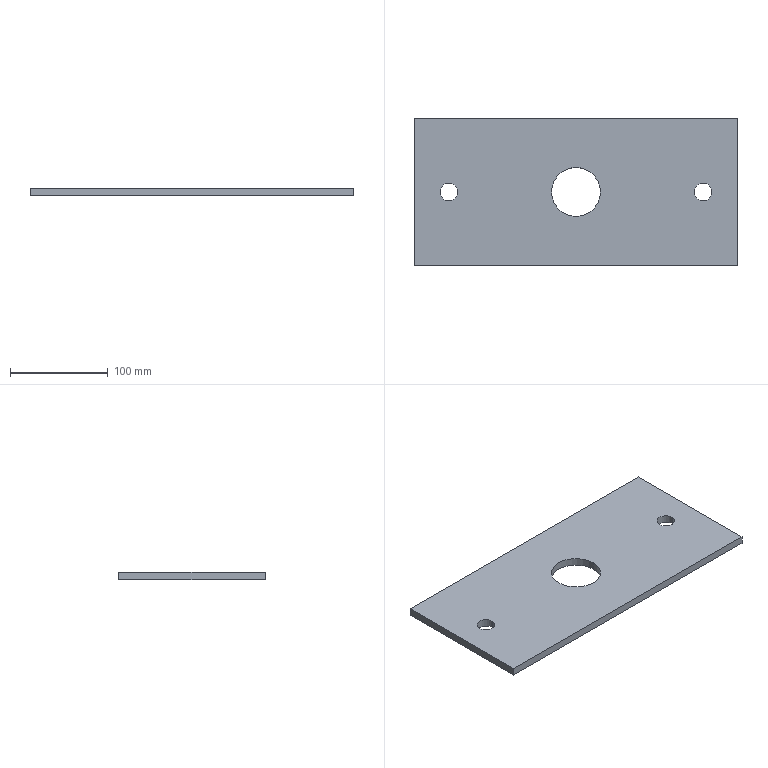Part | STEP file | A_SYL0380DJ1008_1_4-2_CHACHE_AS | 1 solid | 12 faces | box 330 x 150 x 8 mm | volume 376221 mm3 | cylinder 6 | plane 6 | commonest cylinder face diameters 18 x4 50 x2
STEP:
#1=CARTESIAN_POINT('',(25.,0.,0.));
#2=VERTEX_POINT('',#1);
#3=CARTESIAN_POINT('',(25.,0.,8.));
#4=VERTEX_POINT('',#3);
#5=CARTESIAN_POINT('',(25.,0.,0.));
#6=DIRECTION('',(0.,0.,1.));
#7=VECTOR('',#6,1000.);
#8=LINE('',#5,#7);
#9=EDGE_CURVE('',#2,#4,#8,.T.);
#10=ORIENTED_EDGE('',*,*,#9,.F.);
#11=CARTESIAN_POINT('',(-25.,0.,0.));
#12=VERTEX_POINT('',#11);
#13=CARTESIAN_POINT('',(0.,0.,0.));
#14=DIRECTION('',(0.,0.,1.));
#15=DIRECTION('',(-1.,0.,0.));
#16=AXIS2_PLACEMENT_3D('',#13,#14,#15);
#17=CIRCLE('',#16,25.);
#18=EDGE_CURVE('',#12,#2,#17,.T.);
#19=ORIENTED_EDGE('',*,*,#18,.F.);
#20=CARTESIAN_POINT('',(-25.,0.,8.));
#21=VERTEX_POINT('',#20);
#22=CARTESIAN_POINT('',(-25.,0.,0.));
#23=DIRECTION('',(0.,0.,1.));
#24=VECTOR('',#23,1000.);
#25=LINE('',#22,#24);
#26=EDGE_CURVE('',#12,#21,#25,.T.);
#27=ORIENTED_EDGE('',*,*,#26,.T.);
#28=CARTESIAN_POINT('',(0.,0.,8.));
#29=DIRECTION('',(0.,0.,-1.));
#30=DIRECTION('',(1.,0.,0.));
#31=AXIS2_PLACEMENT_3D('',#28,#29,#30);
#32=CIRCLE('',#31,25.);
#33=EDGE_CURVE('',#4,#21,#32,.T.);
#34=ORIENTED_EDGE('',*,*,#33,.F.);
#35=EDGE_LOOP('',(#10,#19,#27,#34));
#36=FACE_OUTER_BOUND('',#35,.T.);
#37=CARTESIAN_POINT('',(0.,0.,4.));
#38=DIRECTION('',(0.,0.,-1.));
#39=DIRECTION('',(-1.,0.,0.));
#40=AXIS2_PLACEMENT_3D('',#37,#38,#39);
#41=CYLINDRICAL_SURFACE('',#40,25.);
#42=ADVANCED_FACE('',(#36),#41,.F.);
#43=CARTESIAN_POINT('',(0.,0.,8.));
#44=DIRECTION('',(0.,0.,-1.));
#45=DIRECTION('',(-1.,0.,0.));
#46=AXIS2_PLACEMENT_3D('',#43,#44,#45);
#47=CIRCLE('',#46,25.);
#48=EDGE_CURVE('',#21,#4,#47,.T.);
#49=ORIENTED_EDGE('',*,*,#48,.F.);
#50=ORIENTED_EDGE('',*,*,#26,.F.);
#51=CARTESIAN_POINT('',(0.,0.,0.));
#52=DIRECTION('',(0.,0.,1.));
#53=DIRECTION('',(1.,0.,0.));
#54=AXIS2_PLACEMENT_3D('',#51,#52,#53);
#55=CIRCLE('',#54,25.);
#56=EDGE_CURVE('',#2,#12,#55,.T.);
#57=ORIENTED_EDGE('',*,*,#56,.F.);
#58=ORIENTED_EDGE('',*,*,#9,.T.);
#59=EDGE_LOOP('',(#49,#50,#57,#58));
#60=FACE_OUTER_BOUND('',#59,.T.);
#61=CARTESIAN_POINT('',(0.,0.,4.));
#62=DIRECTION('',(0.,0.,-1.));
#63=DIRECTION('',(-1.,0.,0.));
#64=AXIS2_PLACEMENT_3D('',#61,#62,#63);
#65=CYLINDRICAL_SURFACE('',#64,25.);
#66=ADVANCED_FACE('',(#60),#65,.F.);
#67=CARTESIAN_POINT('',(-121.,0.,0.));
#68=VERTEX_POINT('',#67);
#69=CARTESIAN_POINT('',(-121.,0.,8.));
#70=VERTEX_POINT('',#69);
#71=CARTESIAN_POINT('',(-121.,0.,0.));
#72=DIRECTION('',(0.,0.,1.));
#73=VECTOR('',#72,1000.);
#74=LINE('',#71,#73);
#75=EDGE_CURVE('',#68,#70,#74,.T.);
#76=ORIENTED_EDGE('',*,*,#75,.F.);
#77=CARTESIAN_POINT('',(-139.,0.,0.));
#78=VERTEX_POINT('',#77);
#79=CARTESIAN_POINT('',(-130.,0.,0.));
#80=DIRECTION('',(0.,0.,1.));
#81=DIRECTION('',(-1.,0.,0.));
#82=AXIS2_PLACEMENT_3D('',#79,#80,#81);
#83=CIRCLE('',#82,9.);
#84=EDGE_CURVE('',#78,#68,#83,.T.);
#85=ORIENTED_EDGE('',*,*,#84,.F.);
#86=CARTESIAN_POINT('',(-139.,0.,8.));
#87=VERTEX_POINT('',#86);
#88=CARTESIAN_POINT('',(-139.,0.,0.));
#89=DIRECTION('',(0.,0.,1.));
#90=VECTOR('',#89,1000.);
#91=LINE('',#88,#90);
#92=EDGE_CURVE('',#78,#87,#91,.T.);
#93=ORIENTED_EDGE('',*,*,#92,.T.);
#94=CARTESIAN_POINT('',(-130.,0.,8.));
#95=DIRECTION('',(0.,0.,-1.));
#96=DIRECTION('',(1.,0.,0.));
#97=AXIS2_PLACEMENT_3D('',#94,#95,#96);
#98=CIRCLE('',#97,9.);
#99=EDGE_CURVE('',#70,#87,#98,.T.);
#100=ORIENTED_EDGE('',*,*,#99,.F.);
#101=EDGE_LOOP('',(#76,#85,#93,#100));
#102=FACE_OUTER_BOUND('',#101,.T.);
#103=CARTESIAN_POINT('',(-130.,0.,4.));
#104=DIRECTION('',(0.,0.,-1.));
#105=DIRECTION('',(-1.,0.,0.));
#106=AXIS2_PLACEMENT_3D('',#103,#104,#105);
#107=CYLINDRICAL_SURFACE('',#106,9.);
#108=ADVANCED_FACE('',(#102),#107,.F.);
#109=CARTESIAN_POINT('',(-130.,0.,8.));
#110=DIRECTION('',(0.,0.,-1.));
#111=DIRECTION('',(-1.,0.,0.));
#112=AXIS2_PLACEMENT_3D('',#109,#110,#111);
#113=CIRCLE('',#112,9.);
#114=EDGE_CURVE('',#87,#70,#113,.T.);
#115=ORIENTED_EDGE('',*,*,#114,.F.);
#116=ORIENTED_EDGE('',*,*,#92,.F.);
#117=CARTESIAN_POINT('',(-130.,0.,0.));
#118=DIRECTION('',(0.,0.,1.));
#119=DIRECTION('',(1.,0.,0.));
#120=AXIS2_PLACEMENT_3D('',#117,#118,#119);
#121=CIRCLE('',#120,9.);
#122=EDGE_CURVE('',#68,#78,#121,.T.);
#123=ORIENTED_EDGE('',*,*,#122,.F.);
#124=ORIENTED_EDGE('',*,*,#75,.T.);
#125=EDGE_LOOP('',(#115,#116,#123,#124));
#126=FACE_OUTER_BOUND('',#125,.T.);
#127=CARTESIAN_POINT('',(-130.,0.,4.));
#128=DIRECTION('',(0.,0.,-1.));
#129=DIRECTION('',(-1.,0.,0.));
#130=AXIS2_PLACEMENT_3D('',#127,#128,#129);
#131=CYLINDRICAL_SURFACE('',#130,9.);
#132=ADVANCED_FACE('',(#126),#131,.F.);
#133=ORIENTED_EDGE('',*,*,#18,.T.);
#134=ORIENTED_EDGE('',*,*,#56,.T.);
#135=EDGE_LOOP('',(#133,#134));
#136=FACE_BOUND('',#135,.T.);
#137=CARTESIAN_POINT('',(121.,0.,0.));
#138=VERTEX_POINT('',#137);
#139=CARTESIAN_POINT('',(139.,0.,0.));
#140=VERTEX_POINT('',#139);
#141=CARTESIAN_POINT('',(130.,0.,0.));
#142=DIRECTION('',(0.,0.,1.));
#143=DIRECTION('',(-1.,0.,0.));
#144=AXIS2_PLACEMENT_3D('',#141,#142,#143);
#145=CIRCLE('',#144,9.);
#146=EDGE_CURVE('',#138,#140,#145,.T.);
#147=ORIENTED_EDGE('',*,*,#146,.T.);
#148=CARTESIAN_POINT('',(130.,0.,0.));
#149=DIRECTION('',(0.,0.,1.));
#150=DIRECTION('',(1.,0.,0.));
#151=AXIS2_PLACEMENT_3D('',#148,#149,#150);
#152=CIRCLE('',#151,9.);
#153=EDGE_CURVE('',#140,#138,#152,.T.);
#154=ORIENTED_EDGE('',*,*,#153,.T.);
#155=EDGE_LOOP('',(#147,#154));
#156=FACE_BOUND('',#155,.T.);
#157=ORIENTED_EDGE('',*,*,#84,.T.);
#158=ORIENTED_EDGE('',*,*,#122,.T.);
#159=EDGE_LOOP('',(#157,#158));
#160=FACE_BOUND('',#159,.T.);
#161=CARTESIAN_POINT('',(165.,-75.,0.));
#162=VERTEX_POINT('',#161);
#163=CARTESIAN_POINT('',(-165.,-75.,0.));
#164=VERTEX_POINT('',#163);
#165=CARTESIAN_POINT('',(165.,-75.,0.));
#166=DIRECTION('',(-1.,0.,0.));
#167=VECTOR('',#166,1000.);
#168=LINE('',#165,#167);
#169=EDGE_CURVE('',#162,#164,#168,.T.);
#170=ORIENTED_EDGE('',*,*,#169,.T.);
#171=CARTESIAN_POINT('',(-165.,75.,0.));
#172=VERTEX_POINT('',#171);
#173=CARTESIAN_POINT('',(-165.,-75.,0.));
#174=DIRECTION('',(0.,1.,0.));
#175=VECTOR('',#174,1000.);
#176=LINE('',#173,#175);
#177=EDGE_CURVE('',#164,#172,#176,.T.);
#178=ORIENTED_EDGE('',*,*,#177,.T.);
#179=CARTESIAN_POINT('',(165.,75.,0.));
#180=VERTEX_POINT('',#179);
#181=CARTESIAN_POINT('',(-165.,75.,0.));
#182=DIRECTION('',(1.,0.,0.));
#183=VECTOR('',#182,1000.);
#184=LINE('',#181,#183);
#185=EDGE_CURVE('',#172,#180,#184,.T.);
#186=ORIENTED_EDGE('',*,*,#185,.T.);
#187=CARTESIAN_POINT('',(165.,75.,0.));
#188=DIRECTION('',(0.,-1.,0.));
#189=VECTOR('',#188,1000.);
#190=LINE('',#187,#189);
#191=EDGE_CURVE('',#180,#162,#190,.T.);
#192=ORIENTED_EDGE('',*,*,#191,.T.);
#193=EDGE_LOOP('',(#170,#178,#186,#192));
#194=FACE_OUTER_BOUND('',#193,.T.);
#195=CARTESIAN_POINT('',(0.,0.,0.));
#196=DIRECTION('',(0.,0.,1.));
#197=DIRECTION('',(1.,0.,0.));
#198=AXIS2_PLACEMENT_3D('',#195,#196,#197);
#199=PLANE('',#198);
#200=ADVANCED_FACE('',(#136,#156,#160,#194),#199,.F.);
#201=CARTESIAN_POINT('',(165.,-75.,8.));
#202=VERTEX_POINT('',#201);
#203=CARTESIAN_POINT('',(165.,-75.,8.));
#204=DIRECTION('',(0.,0.,-1.));
#205=VECTOR('',#204,1000.);
#206=LINE('',#203,#205);
#207=EDGE_CURVE('',#202,#162,#206,.T.);
#208=ORIENTED_EDGE('',*,*,#207,.T.);
#209=ORIENTED_EDGE('',*,*,#191,.F.);
#210=CARTESIAN_POINT('',(165.,75.,8.));
#211=VERTEX_POINT('',#210);
#212=CARTESIAN_POINT('',(165.,75.,8.));
#213=DIRECTION('',(0.,0.,-1.));
#214=VECTOR('',#213,1000.);
#215=LINE('',#212,#214);
#216=EDGE_CURVE('',#211,#180,#215,.T.);
#217=ORIENTED_EDGE('',*,*,#216,.F.);
#218=CARTESIAN_POINT('',(165.,75.,8.));
#219=DIRECTION('',(0.,-1.,0.));
#220=VECTOR('',#219,1000.);
#221=LINE('',#218,#220);
#222=EDGE_CURVE('',#211,#202,#221,.T.);
#223=ORIENTED_EDGE('',*,*,#222,.T.);
#224=EDGE_LOOP('',(#208,#209,#217,#223));
#225=FACE_OUTER_BOUND('',#224,.T.);
#226=CARTESIAN_POINT('',(165.,0.,4.));
#227=DIRECTION('',(-1.,0.,0.));
#228=DIRECTION('',(0.,0.,1.));
#229=AXIS2_PLACEMENT_3D('',#226,#227,#228);
#230=PLANE('',#229);
#231=ADVANCED_FACE('',(#225),#230,.F.);
#232=CARTESIAN_POINT('',(-165.,-75.,8.));
#233=VERTEX_POINT('',#232);
#234=CARTESIAN_POINT('',(-165.,-75.,8.));
#235=DIRECTION('',(0.,0.,-1.));
#236=VECTOR('',#235,1000.);
#237=LINE('',#234,#236);
#238=EDGE_CURVE('',#233,#164,#237,.T.);
#239=ORIENTED_EDGE('',*,*,#238,.T.);
#240=ORIENTED_EDGE('',*,*,#169,.F.);
#241=ORIENTED_EDGE('',*,*,#207,.F.);
#242=CARTESIAN_POINT('',(165.,-75.,8.));
#243=DIRECTION('',(-1.,0.,0.));
#244=VECTOR('',#243,1000.);
#245=LINE('',#242,#244);
#246=EDGE_CURVE('',#202,#233,#245,.T.);
#247=ORIENTED_EDGE('',*,*,#246,.T.);
#248=EDGE_LOOP('',(#239,#240,#241,#247));
#249=FACE_OUTER_BOUND('',#248,.T.);
#250=CARTESIAN_POINT('',(0.,-75.,4.));
#251=DIRECTION('',(0.,1.,0.));
#252=DIRECTION('',(1.,0.,0.));
#253=AXIS2_PLACEMENT_3D('',#250,#251,#252);
#254=PLANE('',#253);
#255=ADVANCED_FACE('',(#249),#254,.F.);
#256=CARTESIAN_POINT('',(-165.,75.,8.));
#257=VERTEX_POINT('',#256);
#258=CARTESIAN_POINT('',(-165.,75.,0.));
#259=DIRECTION('',(0.,0.,1.));
#260=VECTOR('',#259,1000.);
#261=LINE('',#258,#260);
#262=EDGE_CURVE('',#172,#257,#261,.T.);
#263=ORIENTED_EDGE('',*,*,#262,.F.);
#264=ORIENTED_EDGE('',*,*,#177,.F.);
#265=ORIENTED_EDGE('',*,*,#238,.F.);
#266=CARTESIAN_POINT('',(-165.,-75.,8.));
#267=DIRECTION('',(0.,1.,0.));
#268=VECTOR('',#267,1000.);
#269=LINE('',#266,#268);
#270=EDGE_CURVE('',#233,#257,#269,.T.);
#271=ORIENTED_EDGE('',*,*,#270,.T.);
#272=EDGE_LOOP('',(#263,#264,#265,#271));
#273=FACE_OUTER_BOUND('',#272,.T.);
#274=CARTESIAN_POINT('',(-165.,0.,4.));
#275=DIRECTION('',(1.,0.,0.));
#276=DIRECTION('',(0.,1.,0.));
#277=AXIS2_PLACEMENT_3D('',#274,#275,#276);
#278=PLANE('',#277);
#279=ADVANCED_FACE('',(#273),#278,.F.);
#280=ORIENTED_EDGE('',*,*,#216,.T.);
#281=ORIENTED_EDGE('',*,*,#185,.F.);
#282=ORIENTED_EDGE('',*,*,#262,.T.);
#283=CARTESIAN_POINT('',(-165.,75.,8.));
#284=DIRECTION('',(1.,0.,0.));
#285=VECTOR('',#284,1000.);
#286=LINE('',#283,#285);
#287=EDGE_CURVE('',#257,#211,#286,.T.);
#288=ORIENTED_EDGE('',*,*,#287,.T.);
#289=EDGE_LOOP('',(#280,#281,#282,#288));
#290=FACE_OUTER_BOUND('',#289,.T.);
#291=CARTESIAN_POINT('',(0.,75.,4.));
#292=DIRECTION('',(0.,-1.,0.));
#293=DIRECTION('',(0.,0.,-1.));
#294=AXIS2_PLACEMENT_3D('',#291,#292,#293);
#295=PLANE('',#294);
#296=ADVANCED_FACE('',(#290),#295,.F.);
#297=ORIENTED_EDGE('',*,*,#33,.T.);
#298=ORIENTED_EDGE('',*,*,#48,.T.);
#299=EDGE_LOOP('',(#297,#298));
#300=FACE_BOUND('',#299,.T.);
#301=CARTESIAN_POINT('',(139.,0.,8.));
#302=VERTEX_POINT('',#301);
#303=CARTESIAN_POINT('',(121.,0.,8.));
#304=VERTEX_POINT('',#303);
#305=CARTESIAN_POINT('',(130.,0.,8.));
#306=DIRECTION('',(0.,0.,-1.));
#307=DIRECTION('',(1.,0.,0.));
#308=AXIS2_PLACEMENT_3D('',#305,#306,#307);
#309=CIRCLE('',#308,9.);
#310=EDGE_CURVE('',#302,#304,#309,.T.);
#311=ORIENTED_EDGE('',*,*,#310,.T.);
#312=CARTESIAN_POINT('',(130.,0.,8.));
#313=DIRECTION('',(0.,0.,-1.));
#314=DIRECTION('',(-1.,0.,0.));
#315=AXIS2_PLACEMENT_3D('',#312,#313,#314);
#316=CIRCLE('',#315,9.);
#317=EDGE_CURVE('',#304,#302,#316,.T.);
#318=ORIENTED_EDGE('',*,*,#317,.T.);
#319=EDGE_LOOP('',(#311,#318));
#320=FACE_BOUND('',#319,.T.);
#321=ORIENTED_EDGE('',*,*,#99,.T.);
#322=ORIENTED_EDGE('',*,*,#114,.T.);
#323=EDGE_LOOP('',(#321,#322));
#324=FACE_BOUND('',#323,.T.);
#325=ORIENTED_EDGE('',*,*,#270,.F.);
#326=ORIENTED_EDGE('',*,*,#246,.F.);
#327=ORIENTED_EDGE('',*,*,#222,.F.);
#328=ORIENTED_EDGE('',*,*,#287,.F.);
#329=EDGE_LOOP('',(#325,#326,#327,#328));
#330=FACE_OUTER_BOUND('',#329,.T.);
#331=CARTESIAN_POINT('',(0.,0.,8.));
#332=DIRECTION('',(0.,0.,1.));
#333=DIRECTION('',(1.,0.,0.));
#334=AXIS2_PLACEMENT_3D('',#331,#332,#333);
#335=PLANE('',#334);
#336=ADVANCED_FACE('',(#300,#320,#324,#330),#335,.T.);
#337=CARTESIAN_POINT('',(139.,0.,0.));
#338=DIRECTION('',(0.,0.,1.));
#339=VECTOR('',#338,1000.);
#340=LINE('',#337,#339);
#341=EDGE_CURVE('',#140,#302,#340,.T.);
#342=ORIENTED_EDGE('',*,*,#341,.F.);
#343=ORIENTED_EDGE('',*,*,#146,.F.);
#344=CARTESIAN_POINT('',(121.,0.,0.));
#345=DIRECTION('',(0.,0.,1.));
#346=VECTOR('',#345,1000.);
#347=LINE('',#344,#346);
#348=EDGE_CURVE('',#138,#304,#347,.T.);
#349=ORIENTED_EDGE('',*,*,#348,.T.);
#350=ORIENTED_EDGE('',*,*,#310,.F.);
#351=EDGE_LOOP('',(#342,#343,#349,#350));
#352=FACE_OUTER_BOUND('',#351,.T.);
#353=CARTESIAN_POINT('',(130.,0.,4.));
#354=DIRECTION('',(0.,0.,-1.));
#355=DIRECTION('',(-1.,0.,0.));
#356=AXIS2_PLACEMENT_3D('',#353,#354,#355);
#357=CYLINDRICAL_SURFACE('',#356,9.);
#358=ADVANCED_FACE('',(#352),#357,.F.);
#359=ORIENTED_EDGE('',*,*,#317,.F.);
#360=ORIENTED_EDGE('',*,*,#348,.F.);
#361=ORIENTED_EDGE('',*,*,#153,.F.);
#362=ORIENTED_EDGE('',*,*,#341,.T.);
#363=EDGE_LOOP('',(#359,#360,#361,#362));
#364=FACE_OUTER_BOUND('',#363,.T.);
#365=CARTESIAN_POINT('',(130.,0.,4.));
#366=DIRECTION('',(0.,0.,-1.));
#367=DIRECTION('',(-1.,0.,0.));
#368=AXIS2_PLACEMENT_3D('',#365,#366,#367);
#369=CYLINDRICAL_SURFACE('',#368,9.);
#370=ADVANCED_FACE('',(#364),#369,.F.);
#371=CLOSED_SHELL('',(#42,#66,#108,#132,#200,#231,#255,#279,#296,#336,#358,#370));
#372=MANIFOLD_SOLID_BREP('',#371);
#373=CARTESIAN_POINT('',(0.,0.,0.));
#374=DIRECTION('',(0.,0.,1.));
#375=DIRECTION('',(1.,0.,0.));
#376=AXIS2_PLACEMENT_3D('',#373,#374,#375);
#377=(LENGTH_UNIT()NAMED_UNIT(*)SI_UNIT(.MILLI.,.METRE.));
#378=UNCERTAINTY_MEASURE_WITH_UNIT(LENGTH_MEASURE(0.00001),#377,'','');
#379=(NAMED_UNIT(*)PLANE_ANGLE_UNIT()SI_UNIT($,.RADIAN.));
#380=(NAMED_UNIT(*)SI_UNIT($,.STERADIAN.)SOLID_ANGLE_UNIT());
#381=(GEOMETRIC_REPRESENTATION_CONTEXT(3)GLOBAL_UNCERTAINTY_ASSIGNED_CONTEXT((#378))GLOBAL_UNIT_ASSIGNED_CONTEXT((#377,#379,#380))REPRESENTATION_CONTEXT('',''));
#382=ADVANCED_BREP_SHAPE_REPRESENTATION('',(#372,#376),#381);